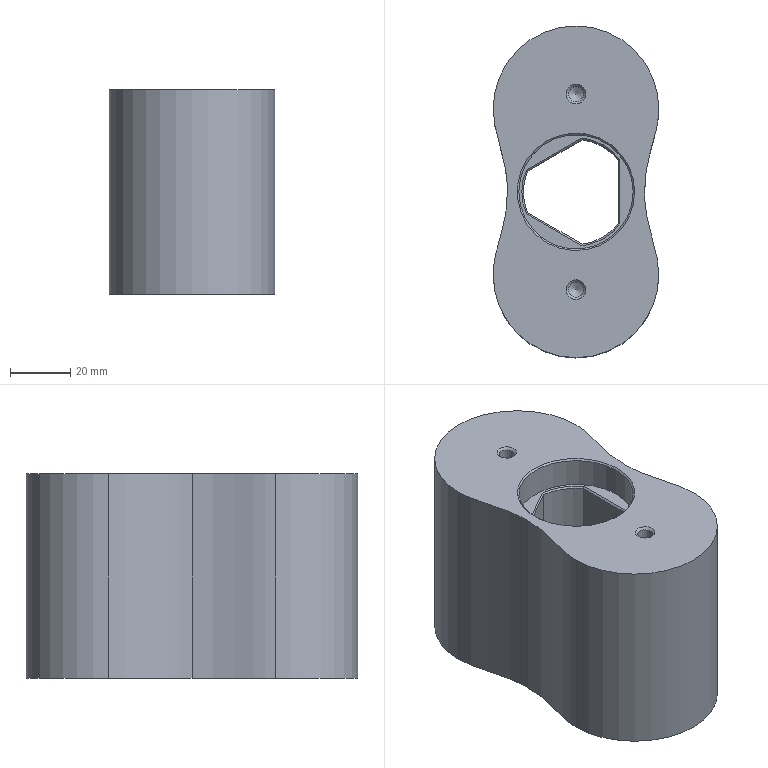Part | 1 solid | 44 faces | box 55.004 x 110.159 x 68 mm | volume 288337 mm3 | cone 16 | plane 13 | cylinder 11 | spline 4 | commonest cylinder face diameters 35 x3 2.5 x2 5 x2 55.004 x2 36.6 x1 38 x1
STEP:
#1=CARTESIAN_POINT('',(-16.093,-6.874,-62.5));
#2=VERTEX_POINT('',#1);
#3=CARTESIAN_POINT('',(-16.093,-6.874,-10.7));
#4=VERTEX_POINT('',#3);
#5=CARTESIAN_POINT('',(-16.093,-6.874,-84.29));
#6=DIRECTION('',(0.,0.,1.));
#7=VECTOR('',#6,1000.);
#8=LINE('',#5,#7);
#9=EDGE_CURVE('',#2,#4,#8,.T.);
#10=ORIENTED_EDGE('',*,*,#9,.F.);
#11=CARTESIAN_POINT('',(-16.093,6.874,-62.5));
#12=VERTEX_POINT('',#11);
#13=CARTESIAN_POINT('',(0.,0.,-62.5));
#14=DIRECTION('',(0.,0.,1.));
#15=DIRECTION('',(1.,0.,0.));
#16=AXIS2_PLACEMENT_3D('',#13,#14,#15);
#17=CIRCLE('',#16,17.5);
#18=EDGE_CURVE('',#2,#12,#17,.F.);
#19=ORIENTED_EDGE('',*,*,#18,.T.);
#20=CARTESIAN_POINT('',(-16.093,6.874,-10.7));
#21=VERTEX_POINT('',#20);
#22=CARTESIAN_POINT('',(-16.093,6.874,-84.29));
#23=DIRECTION('',(0.,0.,1.));
#24=VECTOR('',#23,1000.);
#25=LINE('',#22,#24);
#26=EDGE_CURVE('',#12,#21,#25,.T.);
#27=ORIENTED_EDGE('',*,*,#26,.T.);
#28=CARTESIAN_POINT('',(0.,0.,-10.7));
#29=DIRECTION('',(0.,0.,-1.));
#30=DIRECTION('',(-1.,0.,0.));
#31=AXIS2_PLACEMENT_3D('',#28,#29,#30);
#32=CIRCLE('',#31,17.5);
#33=EDGE_CURVE('',#21,#4,#32,.F.);
#34=ORIENTED_EDGE('',*,*,#33,.T.);
#35=EDGE_LOOP('',(#10,#19,#27,#34));
#36=FACE_BOUND('',#35,.T.);
#37=CARTESIAN_POINT('',(0.,0.,-68.));
#38=DIRECTION('',(0.,0.,-1.));
#39=DIRECTION('',(-1.,0.,0.));
#40=AXIS2_PLACEMENT_3D('',#37,#38,#39);
#41=CYLINDRICAL_SURFACE('',#40,17.5);
#42=ADVANCED_FACE('',(#36),#41,.F.);
#43=CARTESIAN_POINT('',(14.,-10.5,-62.5));
#44=VERTEX_POINT('',#43);
#45=CARTESIAN_POINT('',(14.,-10.5,-10.7));
#46=VERTEX_POINT('',#45);
#47=CARTESIAN_POINT('',(14.,-10.5,-84.29));
#48=DIRECTION('',(0.,0.,1.));
#49=VECTOR('',#48,1000.);
#50=LINE('',#47,#49);
#51=EDGE_CURVE('',#44,#46,#50,.T.);
#52=ORIENTED_EDGE('',*,*,#51,.F.);
#53=CARTESIAN_POINT('',(2.093,-17.374,-62.5));
#54=VERTEX_POINT('',#53);
#55=CARTESIAN_POINT('',(0.,0.,-62.5));
#56=DIRECTION('',(0.,0.,1.));
#57=DIRECTION('',(1.,0.,0.));
#58=AXIS2_PLACEMENT_3D('',#55,#56,#57);
#59=CIRCLE('',#58,17.5);
#60=EDGE_CURVE('',#44,#54,#59,.F.);
#61=ORIENTED_EDGE('',*,*,#60,.T.);
#62=CARTESIAN_POINT('',(2.093,-17.374,-10.7));
#63=VERTEX_POINT('',#62);
#64=CARTESIAN_POINT('',(2.093,-17.374,-84.29));
#65=DIRECTION('',(0.,0.,1.));
#66=VECTOR('',#65,1000.);
#67=LINE('',#64,#66);
#68=EDGE_CURVE('',#54,#63,#67,.T.);
#69=ORIENTED_EDGE('',*,*,#68,.T.);
#70=CARTESIAN_POINT('',(0.,0.,-10.7));
#71=DIRECTION('',(0.,0.,-1.));
#72=DIRECTION('',(-1.,0.,0.));
#73=AXIS2_PLACEMENT_3D('',#70,#71,#72);
#74=CIRCLE('',#73,17.5);
#75=EDGE_CURVE('',#63,#46,#74,.F.);
#76=ORIENTED_EDGE('',*,*,#75,.T.);
#77=EDGE_LOOP('',(#52,#61,#69,#76));
#78=FACE_BOUND('',#77,.T.);
#79=CARTESIAN_POINT('',(0.,0.,-68.));
#80=DIRECTION('',(0.,0.,-1.));
#81=DIRECTION('',(-1.,0.,0.));
#82=AXIS2_PLACEMENT_3D('',#79,#80,#81);
#83=CYLINDRICAL_SURFACE('',#82,17.5);
#84=ADVANCED_FACE('',(#78),#83,.F.);
#85=CARTESIAN_POINT('',(22.771,0.,-68.));
#86=VERTEX_POINT('',#85);
#87=CARTESIAN_POINT('',(27.502,27.577,-68.));
#88=VERTEX_POINT('',#87);
#89=CARTESIAN_POINT('',(22.771,0.,-68.));
#90=CARTESIAN_POINT('',(22.774,2.342,-68.));
#91=CARTESIAN_POINT('',(23.15,7.01,-68.));
#92=CARTESIAN_POINT('',(24.739,13.854,-68.));
#93=CARTESIAN_POINT('',(26.839,20.572,-68.));
#94=CARTESIAN_POINT('',(27.5,25.2,-68.));
#95=CARTESIAN_POINT('',(27.502,27.577,-68.));
#96=B_SPLINE_CURVE_WITH_KNOTS('',3,(#89,#90,#91,#92,#93,#94,#95),.UNSPECIFIED.,.F.,.F.,(4,1,1,1,4),(0.,0.007005,0.01401,0.02102,0.02802),.UNSPECIFIED.);
#97=EDGE_CURVE('',#86,#88,#96,.T.);
#98=ORIENTED_EDGE('',*,*,#97,.T.);
#99=CARTESIAN_POINT('',(27.502,27.577,0.));
#100=VERTEX_POINT('',#99);
#101=CARTESIAN_POINT('',(27.502,27.577,0.));
#102=CARTESIAN_POINT('',(27.502,27.577,-22.667));
#103=CARTESIAN_POINT('',(27.502,27.577,-45.333));
#104=CARTESIAN_POINT('',(27.502,27.577,-68.));
#105=B_SPLINE_CURVE_WITH_KNOTS('',3,(#101,#102,#103,#104),.UNSPECIFIED.,.F.,.F.,(4,4),(0.,1.),.UNSPECIFIED.);
#106=EDGE_CURVE('',#100,#88,#105,.T.);
#107=ORIENTED_EDGE('',*,*,#106,.F.);
#108=CARTESIAN_POINT('',(22.771,0.,0.));
#109=VERTEX_POINT('',#108);
#110=CARTESIAN_POINT('',(22.771,0.,0.));
#111=CARTESIAN_POINT('',(22.774,2.342,0.));
#112=CARTESIAN_POINT('',(23.15,7.01,0.));
#113=CARTESIAN_POINT('',(24.739,13.854,0.));
#114=CARTESIAN_POINT('',(26.839,20.572,0.));
#115=CARTESIAN_POINT('',(27.5,25.2,0.));
#116=CARTESIAN_POINT('',(27.502,27.577,0.));
#117=B_SPLINE_CURVE_WITH_KNOTS('',3,(#110,#111,#112,#113,#114,#115,#116),.UNSPECIFIED.,.F.,.F.,(4,1,1,1,4),(0.,0.007005,0.01401,0.02102,0.02802),.UNSPECIFIED.);
#118=EDGE_CURVE('',#109,#100,#117,.T.);
#119=ORIENTED_EDGE('',*,*,#118,.F.);
#120=CARTESIAN_POINT('',(22.771,0.,0.));
#121=DIRECTION('',(0.,0.,-1.));
#122=VECTOR('',#121,1000.);
#123=LINE('',#120,#122);
#124=EDGE_CURVE('',#109,#86,#123,.T.);
#125=ORIENTED_EDGE('',*,*,#124,.T.);
#126=EDGE_LOOP('',(#98,#107,#119,#125));
#127=FACE_BOUND('',#126,.T.);
#128=CARTESIAN_POINT('',(22.771,0.,0.));
#129=CARTESIAN_POINT('',(22.771,0.,-68.));
#130=CARTESIAN_POINT('',(22.774,2.34,0.));
#131=CARTESIAN_POINT('',(22.774,2.34,-68.));
#132=CARTESIAN_POINT('',(23.153,7.034,0.));
#133=CARTESIAN_POINT('',(23.153,7.034,-68.));
#134=CARTESIAN_POINT('',(24.749,13.889,0.));
#135=CARTESIAN_POINT('',(24.749,13.889,-68.));
#136=CARTESIAN_POINT('',(26.848,20.598,0.));
#137=CARTESIAN_POINT('',(26.848,20.598,-68.));
#138=CARTESIAN_POINT('',(27.5,25.237,0.));
#139=CARTESIAN_POINT('',(27.5,25.237,-68.));
#140=CARTESIAN_POINT('',(27.502,27.577,0.));
#141=CARTESIAN_POINT('',(27.502,27.577,-68.));
#142=B_SPLINE_SURFACE_WITH_KNOTS('',3,1,((#128,#129),(#130,#131),(#132,#133),(#134,#135),(#136,#137),(#138,#139),(#140,#141)),.SURF_OF_LINEAR_EXTRUSION.,.F.,.F.,.F.,(4,1,1,1,4),(2,2),(-0.000004078,0.25,0.5,0.75,1.),(0.,1.),.UNSPECIFIED.);
#143=ADVANCED_FACE('',(#127),#142,.F.);
#144=CARTESIAN_POINT('',(-27.502,27.577,-68.));
#145=VERTEX_POINT('',#144);
#146=CARTESIAN_POINT('',(0.,27.577,-68.));
#147=DIRECTION('',(0.,0.,1.));
#148=DIRECTION('',(1.,0.,0.));
#149=AXIS2_PLACEMENT_3D('',#146,#147,#148);
#150=CIRCLE('',#149,27.502);
#151=EDGE_CURVE('',#88,#145,#150,.T.);
#152=ORIENTED_EDGE('',*,*,#151,.T.);
#153=CARTESIAN_POINT('',(-27.502,27.577,0.));
#154=VERTEX_POINT('',#153);
#155=CARTESIAN_POINT('',(-27.502,27.577,-68.));
#156=CARTESIAN_POINT('',(-27.502,27.577,-45.333));
#157=CARTESIAN_POINT('',(-27.502,27.577,-22.667));
#158=CARTESIAN_POINT('',(-27.502,27.577,0.));
#159=B_SPLINE_CURVE_WITH_KNOTS('',3,(#155,#156,#157,#158),.UNSPECIFIED.,.F.,.F.,(4,4),(0.,1.),.UNSPECIFIED.);
#160=EDGE_CURVE('',#154,#145,#159,.F.);
#161=ORIENTED_EDGE('',*,*,#160,.F.);
#162=CARTESIAN_POINT('',(0.,27.577,0.));
#163=DIRECTION('',(0.,0.,1.));
#164=DIRECTION('',(1.,0.,0.));
#165=AXIS2_PLACEMENT_3D('',#162,#163,#164);
#166=CIRCLE('',#165,27.502);
#167=EDGE_CURVE('',#100,#154,#166,.T.);
#168=ORIENTED_EDGE('',*,*,#167,.F.);
#169=ORIENTED_EDGE('',*,*,#106,.T.);
#170=EDGE_LOOP('',(#152,#161,#168,#169));
#171=FACE_BOUND('',#170,.T.);
#172=CARTESIAN_POINT('',(0.,27.577,0.));
#173=DIRECTION('',(0.,0.,-1.));
#174=DIRECTION('',(-1.,0.,0.));
#175=AXIS2_PLACEMENT_3D('',#172,#173,#174);
#176=CYLINDRICAL_SURFACE('',#175,27.502);
#177=ADVANCED_FACE('',(#171),#176,.T.);
#178=CARTESIAN_POINT('',(-22.771,0.,-68.));
#179=VERTEX_POINT('',#178);
#180=CARTESIAN_POINT('',(-27.502,27.577,-68.));
#181=CARTESIAN_POINT('',(-27.5,25.228,-68.));
#182=CARTESIAN_POINT('',(-26.847,20.595,-68.));
#183=CARTESIAN_POINT('',(-24.741,13.863,-68.));
#184=CARTESIAN_POINT('',(-23.149,7.002,-68.));
#185=CARTESIAN_POINT('',(-22.774,2.348,-68.));
#186=CARTESIAN_POINT('',(-22.771,0.,-68.));
#187=B_SPLINE_CURVE_WITH_KNOTS('',3,(#180,#181,#182,#183,#184,#185,#186),.UNSPECIFIED.,.F.,.F.,(4,1,1,1,4),(0.,0.006997,0.01399,0.02099,0.02799),.UNSPECIFIED.);
#188=EDGE_CURVE('',#145,#179,#187,.T.);
#189=ORIENTED_EDGE('',*,*,#188,.T.);
#190=CARTESIAN_POINT('',(-22.771,0.,0.));
#191=VERTEX_POINT('',#190);
#192=CARTESIAN_POINT('',(-22.771,0.,0.));
#193=DIRECTION('',(0.,0.,-1.));
#194=VECTOR('',#193,1000.);
#195=LINE('',#192,#194);
#196=EDGE_CURVE('',#191,#179,#195,.T.);
#197=ORIENTED_EDGE('',*,*,#196,.F.);
#198=CARTESIAN_POINT('',(-27.502,27.577,0.));
#199=CARTESIAN_POINT('',(-27.5,25.228,0.));
#200=CARTESIAN_POINT('',(-26.847,20.595,0.));
#201=CARTESIAN_POINT('',(-24.741,13.863,0.));
#202=CARTESIAN_POINT('',(-23.149,7.002,0.));
#203=CARTESIAN_POINT('',(-22.774,2.348,0.));
#204=CARTESIAN_POINT('',(-22.771,0.,0.));
#205=B_SPLINE_CURVE_WITH_KNOTS('',3,(#198,#199,#200,#201,#202,#203,#204),.UNSPECIFIED.,.F.,.F.,(4,1,1,1,4),(0.,0.006997,0.01399,0.02099,0.02799),.UNSPECIFIED.);
#206=EDGE_CURVE('',#154,#191,#205,.T.);
#207=ORIENTED_EDGE('',*,*,#206,.F.);
#208=ORIENTED_EDGE('',*,*,#160,.T.);
#209=EDGE_LOOP('',(#189,#197,#207,#208));
#210=FACE_BOUND('',#209,.T.);
#211=CARTESIAN_POINT('',(-27.502,27.577,0.));
#212=CARTESIAN_POINT('',(-27.502,27.577,-68.));
#213=CARTESIAN_POINT('',(-27.5,25.237,0.));
#214=CARTESIAN_POINT('',(-27.5,25.237,-68.));
#215=CARTESIAN_POINT('',(-26.848,20.598,0.));
#216=CARTESIAN_POINT('',(-26.848,20.598,-68.));
#217=CARTESIAN_POINT('',(-24.749,13.889,0.));
#218=CARTESIAN_POINT('',(-24.749,13.889,-68.));
#219=CARTESIAN_POINT('',(-23.153,7.034,0.));
#220=CARTESIAN_POINT('',(-23.153,7.034,-68.));
#221=CARTESIAN_POINT('',(-22.774,2.34,0.));
#222=CARTESIAN_POINT('',(-22.774,2.34,-68.));
#223=CARTESIAN_POINT('',(-22.771,0.,0.));
#224=CARTESIAN_POINT('',(-22.771,0.,-68.));
#225=B_SPLINE_SURFACE_WITH_KNOTS('',3,1,((#211,#212),(#213,#214),(#215,#216),(#217,#218),(#219,#220),(#221,#222),(#223,#224)),.SURF_OF_LINEAR_EXTRUSION.,.F.,.F.,.F.,(4,1,1,1,4),(2,2),(0.,0.25,0.5,0.75,1.),(0.,1.),.UNSPECIFIED.);
#226=ADVANCED_FACE('',(#210),#225,.F.);
#227=CARTESIAN_POINT('',(-27.502,-27.577,-68.));
#228=VERTEX_POINT('',#227);
#229=CARTESIAN_POINT('',(-22.771,0.,-68.));
#230=CARTESIAN_POINT('',(-22.774,-2.342,-68.));
#231=CARTESIAN_POINT('',(-23.15,-7.01,-68.));
#232=CARTESIAN_POINT('',(-24.739,-13.854,-68.));
#233=CARTESIAN_POINT('',(-26.839,-20.572,-68.));
#234=CARTESIAN_POINT('',(-27.5,-25.2,-68.));
#235=CARTESIAN_POINT('',(-27.502,-27.577,-68.));
#236=B_SPLINE_CURVE_WITH_KNOTS('',3,(#229,#230,#231,#232,#233,#234,#235),.UNSPECIFIED.,.F.,.F.,(4,1,1,1,4),(0.,0.007005,0.01401,0.02102,0.02802),.UNSPECIFIED.);
#237=EDGE_CURVE('',#179,#228,#236,.T.);
#238=ORIENTED_EDGE('',*,*,#237,.T.);
#239=CARTESIAN_POINT('',(-27.502,-27.577,0.));
#240=VERTEX_POINT('',#239);
#241=CARTESIAN_POINT('',(-27.502,-27.577,0.));
#242=CARTESIAN_POINT('',(-27.502,-27.577,-22.667));
#243=CARTESIAN_POINT('',(-27.502,-27.577,-45.333));
#244=CARTESIAN_POINT('',(-27.502,-27.577,-68.));
#245=B_SPLINE_CURVE_WITH_KNOTS('',3,(#241,#242,#243,#244),.UNSPECIFIED.,.F.,.F.,(4,4),(0.,1.),.UNSPECIFIED.);
#246=EDGE_CURVE('',#240,#228,#245,.T.);
#247=ORIENTED_EDGE('',*,*,#246,.F.);
#248=CARTESIAN_POINT('',(-22.771,0.,0.));
#249=CARTESIAN_POINT('',(-22.774,-2.342,0.));
#250=CARTESIAN_POINT('',(-23.15,-7.01,0.));
#251=CARTESIAN_POINT('',(-24.739,-13.854,0.));
#252=CARTESIAN_POINT('',(-26.839,-20.572,0.));
#253=CARTESIAN_POINT('',(-27.5,-25.2,0.));
#254=CARTESIAN_POINT('',(-27.502,-27.577,0.));
#255=B_SPLINE_CURVE_WITH_KNOTS('',3,(#248,#249,#250,#251,#252,#253,#254),.UNSPECIFIED.,.F.,.F.,(4,1,1,1,4),(0.,0.007005,0.01401,0.02102,0.02802),.UNSPECIFIED.);
#256=EDGE_CURVE('',#191,#240,#255,.T.);
#257=ORIENTED_EDGE('',*,*,#256,.F.);
#258=ORIENTED_EDGE('',*,*,#196,.T.);
#259=EDGE_LOOP('',(#238,#247,#257,#258));
#260=FACE_BOUND('',#259,.T.);
#261=CARTESIAN_POINT('',(-22.771,0.,0.));
#262=CARTESIAN_POINT('',(-22.771,0.,-68.));
#263=CARTESIAN_POINT('',(-22.774,-2.34,0.));
#264=CARTESIAN_POINT('',(-22.774,-2.34,-68.));
#265=CARTESIAN_POINT('',(-23.153,-7.034,0.));
#266=CARTESIAN_POINT('',(-23.153,-7.034,-68.));
#267=CARTESIAN_POINT('',(-24.749,-13.889,0.));
#268=CARTESIAN_POINT('',(-24.749,-13.889,-68.));
#269=CARTESIAN_POINT('',(-26.848,-20.598,0.));
#270=CARTESIAN_POINT('',(-26.848,-20.598,-68.));
#271=CARTESIAN_POINT('',(-27.5,-25.237,0.));
#272=CARTESIAN_POINT('',(-27.5,-25.237,-68.));
#273=CARTESIAN_POINT('',(-27.502,-27.577,0.));
#274=CARTESIAN_POINT('',(-27.502,-27.577,-68.));
#275=B_SPLINE_SURFACE_WITH_KNOTS('',3,1,((#261,#262),(#263,#264),(#265,#266),(#267,#268),(#269,#270),(#271,#272),(#273,#274)),.SURF_OF_LINEAR_EXTRUSION.,.F.,.F.,.F.,(4,1,1,1,4),(2,2),(-0.000004078,0.25,0.5,0.75,1.),(0.,1.),.UNSPECIFIED.);
#276=ADVANCED_FACE('',(#260),#275,.F.);
#277=CARTESIAN_POINT('',(27.502,-27.577,-68.));
#278=VERTEX_POINT('',#277);
#279=CARTESIAN_POINT('',(0.,-27.577,-68.));
#280=DIRECTION('',(0.,0.,1.));
#281=DIRECTION('',(1.,0.,0.));
#282=AXIS2_PLACEMENT_3D('',#279,#280,#281);
#283=CIRCLE('',#282,27.502);
#284=EDGE_CURVE('',#228,#278,#283,.T.);
#285=ORIENTED_EDGE('',*,*,#284,.T.);
#286=CARTESIAN_POINT('',(27.502,-27.577,0.));
#287=VERTEX_POINT('',#286);
#288=CARTESIAN_POINT('',(27.502,-27.577,-68.));
#289=CARTESIAN_POINT('',(27.502,-27.577,-45.333));
#290=CARTESIAN_POINT('',(27.502,-27.577,-22.667));
#291=CARTESIAN_POINT('',(27.502,-27.577,0.));
#292=B_SPLINE_CURVE_WITH_KNOTS('',3,(#288,#289,#290,#291),.UNSPECIFIED.,.F.,.F.,(4,4),(0.,1.),.UNSPECIFIED.);
#293=EDGE_CURVE('',#287,#278,#292,.F.);
#294=ORIENTED_EDGE('',*,*,#293,.F.);
#295=CARTESIAN_POINT('',(0.,-27.577,0.));
#296=DIRECTION('',(0.,0.,1.));
#297=DIRECTION('',(1.,0.,0.));
#298=AXIS2_PLACEMENT_3D('',#295,#296,#297);
#299=CIRCLE('',#298,27.502);
#300=EDGE_CURVE('',#240,#287,#299,.T.);
#301=ORIENTED_EDGE('',*,*,#300,.F.);
#302=ORIENTED_EDGE('',*,*,#246,.T.);
#303=EDGE_LOOP('',(#285,#294,#301,#302));
#304=FACE_BOUND('',#303,.T.);
#305=CARTESIAN_POINT('',(0.,-27.577,0.));
#306=DIRECTION('',(0.,0.,-1.));
#307=DIRECTION('',(-1.,0.,0.));
#308=AXIS2_PLACEMENT_3D('',#305,#306,#307);
#309=CYLINDRICAL_SURFACE('',#308,27.502);
#310=ADVANCED_FACE('',(#304),#309,.T.);
#311=CARTESIAN_POINT('',(27.502,-27.577,-68.));
#312=CARTESIAN_POINT('',(27.5,-25.228,-68.));
#313=CARTESIAN_POINT('',(26.847,-20.595,-68.));
#314=CARTESIAN_POINT('',(24.741,-13.863,-68.));
#315=CARTESIAN_POINT('',(23.149,-7.002,-68.));
#316=CARTESIAN_POINT('',(22.774,-2.348,-68.));
#317=CARTESIAN_POINT('',(22.771,0.,-68.));
#318=B_SPLINE_CURVE_WITH_KNOTS('',3,(#311,#312,#313,#314,#315,#316,#317),.UNSPECIFIED.,.F.,.F.,(4,1,1,1,4),(0.,0.006997,0.01399,0.02099,0.02799),.UNSPECIFIED.);
#319=EDGE_CURVE('',#278,#86,#318,.T.);
#320=ORIENTED_EDGE('',*,*,#319,.T.);
#321=ORIENTED_EDGE('',*,*,#124,.F.);
#322=CARTESIAN_POINT('',(27.502,-27.577,0.));
#323=CARTESIAN_POINT('',(27.5,-25.228,0.));
#324=CARTESIAN_POINT('',(26.847,-20.595,0.));
#325=CARTESIAN_POINT('',(24.741,-13.863,0.));
#326=CARTESIAN_POINT('',(23.149,-7.002,0.));
#327=CARTESIAN_POINT('',(22.774,-2.348,0.));
#328=CARTESIAN_POINT('',(22.771,0.,0.));
#329=B_SPLINE_CURVE_WITH_KNOTS('',3,(#322,#323,#324,#325,#326,#327,#328),.UNSPECIFIED.,.F.,.F.,(4,1,1,1,4),(0.,0.006997,0.01399,0.02099,0.02799),.UNSPECIFIED.);
#330=EDGE_CURVE('',#287,#109,#329,.T.);
#331=ORIENTED_EDGE('',*,*,#330,.F.);
#332=ORIENTED_EDGE('',*,*,#293,.T.);
#333=EDGE_LOOP('',(#320,#321,#331,#332));
#334=FACE_BOUND('',#333,.T.);
#335=CARTESIAN_POINT('',(27.502,-27.577,0.));
#336=CARTESIAN_POINT('',(27.502,-27.577,-68.));
#337=CARTESIAN_POINT('',(27.5,-25.237,0.));
#338=CARTESIAN_POINT('',(27.5,-25.237,-68.));
#339=CARTESIAN_POINT('',(26.848,-20.598,0.));
#340=CARTESIAN_POINT('',(26.848,-20.598,-68.));
#341=CARTESIAN_POINT('',(24.749,-13.889,0.));
#342=CARTESIAN_POINT('',(24.749,-13.889,-68.));
#343=CARTESIAN_POINT('',(23.153,-7.034,0.));
#344=CARTESIAN_POINT('',(23.153,-7.034,-68.));
#345=CARTESIAN_POINT('',(22.774,-2.34,0.));
#346=CARTESIAN_POINT('',(22.774,-2.34,-68.));
#347=CARTESIAN_POINT('',(22.771,0.,0.));
#348=CARTESIAN_POINT('',(22.771,0.,-68.));
#349=B_SPLINE_SURFACE_WITH_KNOTS('',3,1,((#335,#336),(#337,#338),(#339,#340),(#341,#342),(#343,#344),(#345,#346),(#347,#348)),.SURF_OF_LINEAR_EXTRUSION.,.F.,.F.,.F.,(4,1,1,1,4),(2,2),(0.,0.25,0.5,0.75,1.),(0.,1.),.UNSPECIFIED.);
#350=ADVANCED_FACE('',(#334),#349,.F.);
#351=CARTESIAN_POINT('',(3.25,32.5,0.));
#352=VERTEX_POINT('',#351);
#353=CARTESIAN_POINT('',(0.,32.5,0.));
#354=DIRECTION('',(0.,0.,1.));
#355=DIRECTION('',(1.,0.,0.));
#356=AXIS2_PLACEMENT_3D('',#353,#354,#355);
#357=CIRCLE('',#356,3.25);
#358=EDGE_CURVE('',#352,#352,#357,.T.);
#359=ORIENTED_EDGE('',*,*,#358,.F.);
#360=EDGE_LOOP('',(#359));
#361=FACE_BOUND('',#360,.T.);
#362=CARTESIAN_POINT('',(3.25,-32.5,0.));
#363=VERTEX_POINT('',#362);
#364=CARTESIAN_POINT('',(0.,-32.5,0.));
#365=DIRECTION('',(0.,0.,1.));
#366=DIRECTION('',(1.,0.,0.));
#367=AXIS2_PLACEMENT_3D('',#364,#365,#366);
#368=CIRCLE('',#367,3.25);
#369=EDGE_CURVE('',#363,#363,#368,.T.);
#370=ORIENTED_EDGE('',*,*,#369,.F.);
#371=EDGE_LOOP('',(#370));
#372=FACE_BOUND('',#371,.T.);
#373=CARTESIAN_POINT('',(19.5,0.,0.));
#374=VERTEX_POINT('',#373);
#375=CARTESIAN_POINT('',(0.,0.,0.));
#376=DIRECTION('',(0.,0.,1.));
#377=DIRECTION('',(1.,0.,0.));
#378=AXIS2_PLACEMENT_3D('',#375,#376,#377);
#379=CIRCLE('',#378,19.5);
#380=EDGE_CURVE('',#374,#374,#379,.F.);
#381=ORIENTED_EDGE('',*,*,#380,.T.);
#382=EDGE_LOOP('',(#381));
#383=FACE_BOUND('',#382,.T.);
#384=ORIENTED_EDGE('',*,*,#118,.T.);
#385=ORIENTED_EDGE('',*,*,#167,.T.);
#386=ORIENTED_EDGE('',*,*,#206,.T.);
#387=ORIENTED_EDGE('',*,*,#256,.T.);
#388=ORIENTED_EDGE('',*,*,#300,.T.);
#389=ORIENTED_EDGE('',*,*,#330,.T.);
#390=EDGE_LOOP('',(#384,#385,#386,#387,#388,#389));
#391=FACE_BOUND('',#390,.T.);
#392=CARTESIAN_POINT('',(24.905,13.845,0.));
#393=DIRECTION('',(0.,0.,1.));
#394=DIRECTION('',(1.,0.,0.));
#395=AXIS2_PLACEMENT_3D('',#392,#393,#394);
#396=PLANE('',#395);
#397=ADVANCED_FACE('',(#361,#372,#383,#391),#396,.T.);
#398=CARTESIAN_POINT('',(-1.35,20.25,-68.));
#399=VERTEX_POINT('',#398);
#400=CARTESIAN_POINT('',(0.,20.25,-68.));
#401=DIRECTION('',(0.,0.,-1.));
#402=DIRECTION('',(-1.,0.,0.));
#403=AXIS2_PLACEMENT_3D('',#400,#401,#402);
#404=CIRCLE('',#403,1.35);
#405=EDGE_CURVE('',#399,#399,#404,.T.);
#406=ORIENTED_EDGE('',*,*,#405,.F.);
#407=EDGE_LOOP('',(#406));
#408=FACE_BOUND('',#407,.T.);
#409=CARTESIAN_POINT('',(-1.35,-20.25,-68.));
#410=VERTEX_POINT('',#409);
#411=CARTESIAN_POINT('',(0.,-20.25,-68.));
#412=DIRECTION('',(0.,0.,-1.));
#413=DIRECTION('',(-1.,0.,0.));
#414=AXIS2_PLACEMENT_3D('',#411,#412,#413);
#415=CIRCLE('',#414,1.35);
#416=EDGE_CURVE('',#410,#410,#415,.T.);
#417=ORIENTED_EDGE('',*,*,#416,.F.);
#418=EDGE_LOOP('',(#417));
#419=FACE_BOUND('',#418,.T.);
#420=CARTESIAN_POINT('',(18.8,0.,-68.));
#421=VERTEX_POINT('',#420);
#422=CARTESIAN_POINT('',(0.,0.,-68.));
#423=DIRECTION('',(0.,0.,1.));
#424=DIRECTION('',(1.,0.,0.));
#425=AXIS2_PLACEMENT_3D('',#422,#423,#424);
#426=CIRCLE('',#425,18.8);
#427=EDGE_CURVE('',#421,#421,#426,.T.);
#428=ORIENTED_EDGE('',*,*,#427,.T.);
#429=EDGE_LOOP('',(#428));
#430=FACE_BOUND('',#429,.T.);
#431=ORIENTED_EDGE('',*,*,#97,.F.);
#432=ORIENTED_EDGE('',*,*,#319,.F.);
#433=ORIENTED_EDGE('',*,*,#284,.F.);
#434=ORIENTED_EDGE('',*,*,#237,.F.);
#435=ORIENTED_EDGE('',*,*,#188,.F.);
#436=ORIENTED_EDGE('',*,*,#151,.F.);
#437=EDGE_LOOP('',(#431,#432,#433,#434,#435,#436));
#438=FACE_BOUND('',#437,.T.);
#439=CARTESIAN_POINT('',(24.905,13.845,-68.));
#440=DIRECTION('',(0.,0.,1.));
#441=DIRECTION('',(1.,0.,0.));
#442=AXIS2_PLACEMENT_3D('',#439,#440,#441);
#443=PLANE('',#442);
#444=ADVANCED_FACE('',(#408,#419,#430,#438),#443,.F.);
#445=CARTESIAN_POINT('',(19.,0.,-0.5));
#446=VERTEX_POINT('',#445);
#447=CARTESIAN_POINT('',(0.,0.,-0.5));
#448=DIRECTION('',(0.,0.,1.));
#449=DIRECTION('',(1.,0.,0.));
#450=AXIS2_PLACEMENT_3D('',#447,#448,#449);
#451=CIRCLE('',#450,19.);
#452=EDGE_CURVE('',#446,#446,#451,.T.);
#453=ORIENTED_EDGE('',*,*,#452,.T.);
#454=EDGE_LOOP('',(#453));
#455=FACE_BOUND('',#454,.T.);
#456=CARTESIAN_POINT('',(-19.,0.,-10.2));
#457=VERTEX_POINT('',#456);
#458=CARTESIAN_POINT('',(0.,0.,-10.2));
#459=DIRECTION('',(0.,0.,-1.));
#460=DIRECTION('',(-1.,0.,0.));
#461=AXIS2_PLACEMENT_3D('',#458,#459,#460);
#462=CIRCLE('',#461,19.);
#463=EDGE_CURVE('',#457,#457,#462,.T.);
#464=ORIENTED_EDGE('',*,*,#463,.T.);
#465=EDGE_LOOP('',(#464));
#466=FACE_BOUND('',#465,.T.);
#467=CARTESIAN_POINT('',(0.,0.,-68.));
#468=DIRECTION('',(0.,0.,-1.));
#469=DIRECTION('',(-1.,0.,0.));
#470=AXIS2_PLACEMENT_3D('',#467,#468,#469);
#471=CYLINDRICAL_SURFACE('',#470,19.);
#472=ADVANCED_FACE('',(#455,#466),#471,.F.);
#473=CARTESIAN_POINT('',(1.986,-17.89,-10.2));
#474=VERTEX_POINT('',#473);
#475=CARTESIAN_POINT('',(-16.486,-7.225,-10.2));
#476=VERTEX_POINT('',#475);
#477=CARTESIAN_POINT('',(-16.343,-7.307,-10.2));
#478=DIRECTION('',(-0.866,0.5,0.));
#479=VECTOR('',#478,1000.);
#480=LINE('',#477,#479);
#481=EDGE_CURVE('',#474,#476,#480,.T.);
#482=ORIENTED_EDGE('',*,*,#481,.T.);
#483=CARTESIAN_POINT('',(-16.486,7.225,-10.2));
#484=VERTEX_POINT('',#483);
#485=CARTESIAN_POINT('',(0.,0.,-10.2));
#486=DIRECTION('',(0.,0.,-1.));
#487=DIRECTION('',(-1.,0.,0.));
#488=AXIS2_PLACEMENT_3D('',#485,#486,#487);
#489=CIRCLE('',#488,18.);
#490=EDGE_CURVE('',#476,#484,#489,.T.);
#491=ORIENTED_EDGE('',*,*,#490,.T.);
#492=CARTESIAN_POINT('',(1.986,17.89,-10.2));
#493=VERTEX_POINT('',#492);
#494=CARTESIAN_POINT('',(1.843,17.807,-10.2));
#495=DIRECTION('',(0.866,0.5,0.));
#496=VECTOR('',#495,1000.);
#497=LINE('',#494,#496);
#498=EDGE_CURVE('',#484,#493,#497,.T.);
#499=ORIENTED_EDGE('',*,*,#498,.T.);
#500=CARTESIAN_POINT('',(14.5,10.665,-10.2));
#501=VERTEX_POINT('',#500);
#502=CARTESIAN_POINT('',(0.,0.,-10.2));
#503=DIRECTION('',(0.,0.,-1.));
#504=DIRECTION('',(-1.,0.,0.));
#505=AXIS2_PLACEMENT_3D('',#502,#503,#504);
#506=CIRCLE('',#505,18.);
#507=EDGE_CURVE('',#493,#501,#506,.T.);
#508=ORIENTED_EDGE('',*,*,#507,.T.);
#509=CARTESIAN_POINT('',(14.5,-10.665,-10.2));
#510=VERTEX_POINT('',#509);
#511=CARTESIAN_POINT('',(14.5,-10.5,-10.2));
#512=DIRECTION('',(0.,-1.,0.));
#513=VECTOR('',#512,1000.);
#514=LINE('',#511,#513);
#515=EDGE_CURVE('',#501,#510,#514,.T.);
#516=ORIENTED_EDGE('',*,*,#515,.T.);
#517=CARTESIAN_POINT('',(0.,0.,-10.2));
#518=DIRECTION('',(0.,0.,-1.));
#519=DIRECTION('',(-1.,0.,0.));
#520=AXIS2_PLACEMENT_3D('',#517,#518,#519);
#521=CIRCLE('',#520,18.);
#522=EDGE_CURVE('',#510,#474,#521,.T.);
#523=ORIENTED_EDGE('',*,*,#522,.T.);
#524=EDGE_LOOP('',(#482,#491,#499,#508,#516,#523));
#525=FACE_BOUND('',#524,.T.);
#526=ORIENTED_EDGE('',*,*,#463,.F.);
#527=EDGE_LOOP('',(#526));
#528=FACE_BOUND('',#527,.T.);
#529=CARTESIAN_POINT('',(0.,19.,-10.2));
#530=DIRECTION('',(0.,0.,-1.));
#531=DIRECTION('',(-1.,0.,0.));
#532=AXIS2_PLACEMENT_3D('',#529,#530,#531);
#533=PLANE('',#532);
#534=ADVANCED_FACE('',(#525,#528),#533,.F.);
#535=CARTESIAN_POINT('',(2.093,17.374,-62.5));
#536=VERTEX_POINT('',#535);
#537=CARTESIAN_POINT('',(2.093,17.374,-10.7));
#538=VERTEX_POINT('',#537);
#539=CARTESIAN_POINT('',(2.093,17.374,-84.29));
#540=DIRECTION('',(0.,0.,1.));
#541=VECTOR('',#540,1000.);
#542=LINE('',#539,#541);
#543=EDGE_CURVE('',#536,#538,#542,.T.);
#544=ORIENTED_EDGE('',*,*,#543,.F.);
#545=CARTESIAN_POINT('',(14.,10.5,-62.5));
#546=VERTEX_POINT('',#545);
#547=CARTESIAN_POINT('',(0.,0.,-62.5));
#548=DIRECTION('',(0.,0.,1.));
#549=DIRECTION('',(1.,0.,0.));
#550=AXIS2_PLACEMENT_3D('',#547,#548,#549);
#551=CIRCLE('',#550,17.5);
#552=EDGE_CURVE('',#536,#546,#551,.F.);
#553=ORIENTED_EDGE('',*,*,#552,.T.);
#554=CARTESIAN_POINT('',(14.,10.5,-10.7));
#555=VERTEX_POINT('',#554);
#556=CARTESIAN_POINT('',(14.,10.5,-84.29));
#557=DIRECTION('',(0.,0.,1.));
#558=VECTOR('',#557,1000.);
#559=LINE('',#556,#558);
#560=EDGE_CURVE('',#546,#555,#559,.T.);
#561=ORIENTED_EDGE('',*,*,#560,.T.);
#562=CARTESIAN_POINT('',(0.,0.,-10.7));
#563=DIRECTION('',(0.,0.,-1.));
#564=DIRECTION('',(-1.,0.,0.));
#565=AXIS2_PLACEMENT_3D('',#562,#563,#564);
#566=CIRCLE('',#565,17.5);
#567=EDGE_CURVE('',#555,#538,#566,.F.);
#568=ORIENTED_EDGE('',*,*,#567,.T.);
#569=EDGE_LOOP('',(#544,#553,#561,#568));
#570=FACE_BOUND('',#569,.T.);
#571=CARTESIAN_POINT('',(0.,0.,-68.));
#572=DIRECTION('',(0.,0.,-1.));
#573=DIRECTION('',(-1.,0.,0.));
#574=AXIS2_PLACEMENT_3D('',#571,#572,#573);
#575=CYLINDRICAL_SURFACE('',#574,17.5);
#576=ADVANCED_FACE('',(#570),#575,.F.);
#577=CARTESIAN_POINT('',(1.986,17.89,-63.));
#578=VERTEX_POINT('',#577);
#579=CARTESIAN_POINT('',(-16.486,7.225,-63.));
#580=VERTEX_POINT('',#579);
#581=CARTESIAN_POINT('',(-16.343,7.307,-63.));
#582=DIRECTION('',(-0.866,-0.5,0.));
#583=VECTOR('',#582,1000.);
#584=LINE('',#581,#583);
#585=EDGE_CURVE('',#578,#580,#584,.T.);
#586=ORIENTED_EDGE('',*,*,#585,.T.);
#587=CARTESIAN_POINT('',(-16.486,-7.225,-63.));
#588=VERTEX_POINT('',#587);
#589=CARTESIAN_POINT('',(0.,0.,-63.));
#590=DIRECTION('',(0.,0.,1.));
#591=DIRECTION('',(1.,0.,0.));
#592=AXIS2_PLACEMENT_3D('',#589,#590,#591);
#593=CIRCLE('',#592,18.);
#594=EDGE_CURVE('',#580,#588,#593,.T.);
#595=ORIENTED_EDGE('',*,*,#594,.T.);
#596=CARTESIAN_POINT('',(1.986,-17.89,-63.));
#597=VERTEX_POINT('',#596);
#598=CARTESIAN_POINT('',(1.843,-17.807,-63.));
#599=DIRECTION('',(0.866,-0.5,0.));
#600=VECTOR('',#599,1000.);
#601=LINE('',#598,#600);
#602=EDGE_CURVE('',#588,#597,#601,.T.);
#603=ORIENTED_EDGE('',*,*,#602,.T.);
#604=CARTESIAN_POINT('',(14.5,-10.665,-63.));
#605=VERTEX_POINT('',#604);
#606=CARTESIAN_POINT('',(0.,0.,-63.));
#607=DIRECTION('',(0.,0.,1.));
#608=DIRECTION('',(1.,0.,0.));
#609=AXIS2_PLACEMENT_3D('',#606,#607,#608);
#610=CIRCLE('',#609,18.);
#611=EDGE_CURVE('',#597,#605,#610,.T.);
#612=ORIENTED_EDGE('',*,*,#611,.T.);
#613=CARTESIAN_POINT('',(14.5,10.665,-63.));
#614=VERTEX_POINT('',#613);
#615=CARTESIAN_POINT('',(14.5,10.5,-63.));
#616=DIRECTION('',(0.,1.,0.));
#617=VECTOR('',#616,1000.);
#618=LINE('',#615,#617);
#619=EDGE_CURVE('',#605,#614,#618,.T.);
#620=ORIENTED_EDGE('',*,*,#619,.T.);
#621=CARTESIAN_POINT('',(0.,0.,-63.));
#622=DIRECTION('',(0.,0.,1.));
#623=DIRECTION('',(1.,0.,0.));
#624=AXIS2_PLACEMENT_3D('',#621,#622,#623);
#625=CIRCLE('',#624,18.);
#626=EDGE_CURVE('',#614,#578,#625,.T.);
#627=ORIENTED_EDGE('',*,*,#626,.T.);
#628=EDGE_LOOP('',(#586,#595,#603,#612,#620,#627));
#629=FACE_BOUND('',#628,.T.);
#630=CARTESIAN_POINT('',(-18.3,0.,-63.));
#631=VERTEX_POINT('',#630);
#632=CARTESIAN_POINT('',(0.,0.,-63.));
#633=DIRECTION('',(0.,0.,-1.));
#634=DIRECTION('',(-1.,0.,0.));
#635=AXIS2_PLACEMENT_3D('',#632,#633,#634);
#636=CIRCLE('',#635,18.3);
#637=EDGE_CURVE('',#631,#631,#636,.T.);
#638=ORIENTED_EDGE('',*,*,#637,.T.);
#639=EDGE_LOOP('',(#638));
#640=FACE_BOUND('',#639,.T.);
#641=CARTESIAN_POINT('',(0.,17.5,-63.));
#642=DIRECTION('',(0.,0.,1.));
#643=DIRECTION('',(1.,0.,0.));
#644=AXIS2_PLACEMENT_3D('',#641,#642,#643);
#645=PLANE('',#644);
#646=ADVANCED_FACE('',(#629,#640),#645,.F.);
#647=CARTESIAN_POINT('',(18.3,0.,-67.5));
#648=VERTEX_POINT('',#647);
#649=CARTESIAN_POINT('',(0.,0.,-67.5));
#650=DIRECTION('',(0.,0.,1.));
#651=DIRECTION('',(1.,0.,0.));
#652=AXIS2_PLACEMENT_3D('',#649,#650,#651);
#653=CIRCLE('',#652,18.3);
#654=EDGE_CURVE('',#648,#648,#653,.F.);
#655=ORIENTED_EDGE('',*,*,#654,.T.);
#656=EDGE_LOOP('',(#655));
#657=FACE_BOUND('',#656,.T.);
#658=ORIENTED_EDGE('',*,*,#637,.F.);
#659=EDGE_LOOP('',(#658));
#660=FACE_BOUND('',#659,.T.);
#661=CARTESIAN_POINT('',(0.,0.,-68.));
#662=DIRECTION('',(0.,0.,-1.));
#663=DIRECTION('',(-1.,0.,0.));
#664=AXIS2_PLACEMENT_3D('',#661,#662,#663);
#665=CYLINDRICAL_SURFACE('',#664,18.3);
#666=ADVANCED_FACE('',(#657,#660),#665,.F.);
#667=ORIENTED_EDGE('',*,*,#560,.F.);
#668=CARTESIAN_POINT('',(14.,-10.5,-62.5));
#669=DIRECTION('',(0.,-1.,0.));
#670=VECTOR('',#669,1000.);
#671=LINE('',#668,#670);
#672=EDGE_CURVE('',#546,#44,#671,.T.);
#673=ORIENTED_EDGE('',*,*,#672,.T.);
#674=ORIENTED_EDGE('',*,*,#51,.T.);
#675=CARTESIAN_POINT('',(14.,10.5,-10.7));
#676=DIRECTION('',(0.,1.,0.));
#677=VECTOR('',#676,1000.);
#678=LINE('',#675,#677);
#679=EDGE_CURVE('',#46,#555,#678,.T.);
#680=ORIENTED_EDGE('',*,*,#679,.T.);
#681=EDGE_LOOP('',(#667,#673,#674,#680));
#682=FACE_BOUND('',#681,.T.);
#683=CARTESIAN_POINT('',(14.,10.5,-84.29));
#684=DIRECTION('',(-1.,0.,0.));
#685=DIRECTION('',(0.,0.,1.));
#686=AXIS2_PLACEMENT_3D('',#683,#684,#685);
#687=PLANE('',#686);
#688=ADVANCED_FACE('',(#682),#687,.T.);
#689=ORIENTED_EDGE('',*,*,#68,.F.);
#690=CARTESIAN_POINT('',(-16.093,-6.874,-62.5));
#691=DIRECTION('',(-0.866,0.5,0.));
#692=VECTOR('',#691,1000.);
#693=LINE('',#690,#692);
#694=EDGE_CURVE('',#54,#2,#693,.T.);
#695=ORIENTED_EDGE('',*,*,#694,.T.);
#696=ORIENTED_EDGE('',*,*,#9,.T.);
#697=CARTESIAN_POINT('',(2.093,-17.374,-10.7));
#698=DIRECTION('',(0.866,-0.5,0.));
#699=VECTOR('',#698,1000.);
#700=LINE('',#697,#699);
#701=EDGE_CURVE('',#4,#63,#700,.T.);
#702=ORIENTED_EDGE('',*,*,#701,.T.);
#703=EDGE_LOOP('',(#689,#695,#696,#702));
#704=FACE_BOUND('',#703,.T.);
#705=CARTESIAN_POINT('',(2.093,-17.374,-84.29));
#706=DIRECTION('',(0.5,0.866,0.));
#707=DIRECTION('',(-0.866,0.5,0.));
#708=AXIS2_PLACEMENT_3D('',#705,#706,#707);
#709=PLANE('',#708);
#710=ADVANCED_FACE('',(#704),#709,.T.);
#711=ORIENTED_EDGE('',*,*,#26,.F.);
#712=CARTESIAN_POINT('',(2.093,17.374,-62.5));
#713=DIRECTION('',(0.866,0.5,0.));
#714=VECTOR('',#713,1000.);
#715=LINE('',#712,#714);
#716=EDGE_CURVE('',#12,#536,#715,.T.);
#717=ORIENTED_EDGE('',*,*,#716,.T.);
#718=ORIENTED_EDGE('',*,*,#543,.T.);
#719=CARTESIAN_POINT('',(-16.093,6.874,-10.7));
#720=DIRECTION('',(-0.866,-0.5,0.));
#721=VECTOR('',#720,1000.);
#722=LINE('',#719,#721);
#723=EDGE_CURVE('',#538,#21,#722,.T.);
#724=ORIENTED_EDGE('',*,*,#723,.T.);
#725=EDGE_LOOP('',(#711,#717,#718,#724));
#726=FACE_BOUND('',#725,.T.);
#727=CARTESIAN_POINT('',(-16.093,6.874,-84.29));
#728=DIRECTION('',(0.5,-0.866,0.));
#729=DIRECTION('',(0.866,0.5,0.));
#730=AXIS2_PLACEMENT_3D('',#727,#728,#729);
#731=PLANE('',#730);
#732=ADVANCED_FACE('',(#726),#731,.T.);
#733=ORIENTED_EDGE('',*,*,#452,.F.);
#734=EDGE_LOOP('',(#733));
#735=FACE_BOUND('',#734,.T.);
#736=ORIENTED_EDGE('',*,*,#380,.F.);
#737=EDGE_LOOP('',(#736));
#738=FACE_BOUND('',#737,.T.);
#739=CARTESIAN_POINT('',(0.,0.,0.));
#740=DIRECTION('',(0.,0.,1.));
#741=DIRECTION('',(1.,0.,0.));
#742=AXIS2_PLACEMENT_3D('',#739,#740,#741);
#743=CONICAL_SURFACE('',#742,19.5,0.7854);
#744=ADVANCED_FACE('',(#735,#738),#743,.F.);
#745=ORIENTED_EDGE('',*,*,#427,.F.);
#746=EDGE_LOOP('',(#745));
#747=FACE_BOUND('',#746,.T.);
#748=ORIENTED_EDGE('',*,*,#654,.F.);
#749=EDGE_LOOP('',(#748));
#750=FACE_BOUND('',#749,.T.);
#751=CARTESIAN_POINT('',(0.,0.,-67.5));
#752=DIRECTION('',(0.,0.,-1.));
#753=DIRECTION('',(-1.,0.,0.));
#754=AXIS2_PLACEMENT_3D('',#751,#752,#753);
#755=CONICAL_SURFACE('',#754,18.3,0.7854);
#756=ADVANCED_FACE('',(#747,#750),#755,.F.);
#757=CARTESIAN_POINT('',(14.,10.5,-62.5));
#758=CARTESIAN_POINT('',(14.167,10.556,-62.667));
#759=CARTESIAN_POINT('',(14.333,10.611,-62.833));
#760=CARTESIAN_POINT('',(14.5,10.665,-63.));
#761=B_SPLINE_CURVE_WITH_KNOTS('',3,(#757,#758,#759,#760),.UNSPECIFIED.,.F.,.F.,(4,4),(0.,0.0007262),.UNSPECIFIED.);
#762=EDGE_CURVE('',#614,#546,#761,.F.);
#763=ORIENTED_EDGE('',*,*,#762,.F.);
#764=ORIENTED_EDGE('',*,*,#619,.F.);
#765=CARTESIAN_POINT('',(14.,-10.5,-62.5));
#766=CARTESIAN_POINT('',(14.167,-10.556,-62.667));
#767=CARTESIAN_POINT('',(14.333,-10.611,-62.833));
#768=CARTESIAN_POINT('',(14.5,-10.665,-63.));
#769=B_SPLINE_CURVE_WITH_KNOTS('',3,(#765,#766,#767,#768),.UNSPECIFIED.,.F.,.F.,(4,4),(0.,0.0007262),.UNSPECIFIED.);
#770=EDGE_CURVE('',#44,#605,#769,.T.);
#771=ORIENTED_EDGE('',*,*,#770,.F.);
#772=ORIENTED_EDGE('',*,*,#672,.F.);
#773=EDGE_LOOP('',(#763,#764,#771,#772));
#774=FACE_BOUND('',#773,.T.);
#775=CARTESIAN_POINT('',(14.5,17.5,-63.));
#776=DIRECTION('',(-0.7071,0.,-0.7071));
#777=DIRECTION('',(0.,-1.,0.));
#778=AXIS2_PLACEMENT_3D('',#775,#776,#777);
#779=PLANE('',#778);
#780=ADVANCED_FACE('',(#774),#779,.T.);
#781=ORIENTED_EDGE('',*,*,#770,.T.);
#782=ORIENTED_EDGE('',*,*,#611,.F.);
#783=CARTESIAN_POINT('',(2.093,-17.374,-62.5));
#784=CARTESIAN_POINT('',(2.058,-17.546,-62.667));
#785=CARTESIAN_POINT('',(2.022,-17.718,-62.833));
#786=CARTESIAN_POINT('',(1.986,-17.89,-63.));
#787=B_SPLINE_CURVE_WITH_KNOTS('',3,(#783,#784,#785,#786),.UNSPECIFIED.,.F.,.F.,(4,4),(0.,0.0007262),.UNSPECIFIED.);
#788=EDGE_CURVE('',#54,#597,#787,.T.);
#789=ORIENTED_EDGE('',*,*,#788,.F.);
#790=ORIENTED_EDGE('',*,*,#60,.F.);
#791=EDGE_LOOP('',(#781,#782,#789,#790));
#792=FACE_BOUND('',#791,.T.);
#793=CARTESIAN_POINT('',(0.,0.,-62.5));
#794=DIRECTION('',(0.,0.,-1.));
#795=DIRECTION('',(-1.,0.,0.));
#796=AXIS2_PLACEMENT_3D('',#793,#794,#795);
#797=CONICAL_SURFACE('',#796,17.5,0.7854);
#798=ADVANCED_FACE('',(#792),#797,.F.);
#799=ORIENTED_EDGE('',*,*,#762,.T.);
#800=ORIENTED_EDGE('',*,*,#552,.F.);
#801=CARTESIAN_POINT('',(2.093,17.374,-62.5));
#802=CARTESIAN_POINT('',(2.058,17.546,-62.667));
#803=CARTESIAN_POINT('',(2.022,17.718,-62.833));
#804=CARTESIAN_POINT('',(1.986,17.89,-63.));
#805=B_SPLINE_CURVE_WITH_KNOTS('',3,(#801,#802,#803,#804),.UNSPECIFIED.,.F.,.F.,(4,4),(0.,0.0007262),.UNSPECIFIED.);
#806=EDGE_CURVE('',#578,#536,#805,.F.);
#807=ORIENTED_EDGE('',*,*,#806,.F.);
#808=ORIENTED_EDGE('',*,*,#626,.F.);
#809=EDGE_LOOP('',(#799,#800,#807,#808));
#810=FACE_BOUND('',#809,.T.);
#811=CARTESIAN_POINT('',(0.,0.,-62.5));
#812=DIRECTION('',(0.,0.,-1.));
#813=DIRECTION('',(-1.,0.,0.));
#814=AXIS2_PLACEMENT_3D('',#811,#812,#813);
#815=CONICAL_SURFACE('',#814,17.5,0.7854);
#816=ADVANCED_FACE('',(#810),#815,.F.);
#817=ORIENTED_EDGE('',*,*,#788,.T.);
#818=ORIENTED_EDGE('',*,*,#602,.F.);
#819=CARTESIAN_POINT('',(-16.486,-7.225,-63.));
#820=CARTESIAN_POINT('',(-16.356,-7.108,-62.833));
#821=CARTESIAN_POINT('',(-16.225,-6.991,-62.667));
#822=CARTESIAN_POINT('',(-16.093,-6.874,-62.5));
#823=B_SPLINE_CURVE_WITH_KNOTS('',3,(#819,#820,#821,#822),.UNSPECIFIED.,.F.,.F.,(4,4),(0.,0.0007262),.UNSPECIFIED.);
#824=EDGE_CURVE('',#2,#588,#823,.F.);
#825=ORIENTED_EDGE('',*,*,#824,.F.);
#826=ORIENTED_EDGE('',*,*,#694,.F.);
#827=EDGE_LOOP('',(#817,#818,#825,#826));
#828=FACE_BOUND('',#827,.T.);
#829=CARTESIAN_POINT('',(-14.828,-8.182,-63.));
#830=DIRECTION('',(0.3536,0.6124,-0.7071));
#831=DIRECTION('',(-0.866,0.5,0.));
#832=AXIS2_PLACEMENT_3D('',#829,#830,#831);
#833=PLANE('',#832);
#834=ADVANCED_FACE('',(#828),#833,.T.);
#835=ORIENTED_EDGE('',*,*,#806,.T.);
#836=ORIENTED_EDGE('',*,*,#716,.F.);
#837=CARTESIAN_POINT('',(-16.093,6.874,-62.5));
#838=CARTESIAN_POINT('',(-16.225,6.991,-62.667));
#839=CARTESIAN_POINT('',(-16.356,7.108,-62.833));
#840=CARTESIAN_POINT('',(-16.486,7.225,-63.));
#841=B_SPLINE_CURVE_WITH_KNOTS('',3,(#837,#838,#839,#840),.UNSPECIFIED.,.F.,.F.,(4,4),(0.,0.0007262),.UNSPECIFIED.);
#842=EDGE_CURVE('',#580,#12,#841,.F.);
#843=ORIENTED_EDGE('',*,*,#842,.F.);
#844=ORIENTED_EDGE('',*,*,#585,.F.);
#845=EDGE_LOOP('',(#835,#836,#843,#844));
#846=FACE_BOUND('',#845,.T.);
#847=CARTESIAN_POINT('',(0.3277,16.932,-63.));
#848=DIRECTION('',(0.3536,-0.6124,-0.7071));
#849=DIRECTION('',(0.866,0.5,0.));
#850=AXIS2_PLACEMENT_3D('',#847,#848,#849);
#851=PLANE('',#850);
#852=ADVANCED_FACE('',(#846),#851,.T.);
#853=ORIENTED_EDGE('',*,*,#824,.T.);
#854=ORIENTED_EDGE('',*,*,#594,.F.);
#855=ORIENTED_EDGE('',*,*,#842,.T.);
#856=ORIENTED_EDGE('',*,*,#18,.F.);
#857=EDGE_LOOP('',(#853,#854,#855,#856));
#858=FACE_BOUND('',#857,.T.);
#859=CARTESIAN_POINT('',(0.,0.,-62.5));
#860=DIRECTION('',(0.,0.,-1.));
#861=DIRECTION('',(-1.,0.,0.));
#862=AXIS2_PLACEMENT_3D('',#859,#860,#861);
#863=CONICAL_SURFACE('',#862,17.5,0.7854);
#864=ADVANCED_FACE('',(#858),#863,.F.);
#865=CARTESIAN_POINT('',(14.5,10.665,-10.2));
#866=CARTESIAN_POINT('',(14.333,10.611,-10.367));
#867=CARTESIAN_POINT('',(14.167,10.556,-10.533));
#868=CARTESIAN_POINT('',(14.,10.5,-10.7));
#869=B_SPLINE_CURVE_WITH_KNOTS('',3,(#865,#866,#867,#868),.UNSPECIFIED.,.F.,.F.,(4,4),(0.,0.0007262),.UNSPECIFIED.);
#870=EDGE_CURVE('',#555,#501,#869,.F.);
#871=ORIENTED_EDGE('',*,*,#870,.F.);
#872=ORIENTED_EDGE('',*,*,#679,.F.);
#873=CARTESIAN_POINT('',(14.5,-10.665,-10.2));
#874=CARTESIAN_POINT('',(14.333,-10.611,-10.367));
#875=CARTESIAN_POINT('',(14.167,-10.556,-10.533));
#876=CARTESIAN_POINT('',(14.,-10.5,-10.7));
#877=B_SPLINE_CURVE_WITH_KNOTS('',3,(#873,#874,#875,#876),.UNSPECIFIED.,.F.,.F.,(4,4),(0.,0.0007262),.UNSPECIFIED.);
#878=EDGE_CURVE('',#510,#46,#877,.T.);
#879=ORIENTED_EDGE('',*,*,#878,.F.);
#880=ORIENTED_EDGE('',*,*,#515,.F.);
#881=EDGE_LOOP('',(#871,#872,#879,#880));
#882=FACE_BOUND('',#881,.T.);
#883=CARTESIAN_POINT('',(14.5,19.,-10.2));
#884=DIRECTION('',(-0.7071,0.,0.7071));
#885=DIRECTION('',(0.,1.,0.));
#886=AXIS2_PLACEMENT_3D('',#883,#884,#885);
#887=PLANE('',#886);
#888=ADVANCED_FACE('',(#882),#887,.T.);
#889=ORIENTED_EDGE('',*,*,#878,.T.);
#890=ORIENTED_EDGE('',*,*,#75,.F.);
#891=CARTESIAN_POINT('',(1.986,-17.89,-10.2));
#892=CARTESIAN_POINT('',(2.022,-17.718,-10.367));
#893=CARTESIAN_POINT('',(2.058,-17.546,-10.533));
#894=CARTESIAN_POINT('',(2.093,-17.374,-10.7));
#895=B_SPLINE_CURVE_WITH_KNOTS('',3,(#891,#892,#893,#894),.UNSPECIFIED.,.F.,.F.,(4,4),(0.,0.0007262),.UNSPECIFIED.);
#896=EDGE_CURVE('',#474,#63,#895,.T.);
#897=ORIENTED_EDGE('',*,*,#896,.F.);
#898=ORIENTED_EDGE('',*,*,#522,.F.);
#899=EDGE_LOOP('',(#889,#890,#897,#898));
#900=FACE_BOUND('',#899,.T.);
#901=CARTESIAN_POINT('',(0.,0.,-10.2));
#902=DIRECTION('',(0.,0.,1.));
#903=DIRECTION('',(1.,0.,0.));
#904=AXIS2_PLACEMENT_3D('',#901,#902,#903);
#905=CONICAL_SURFACE('',#904,18.,0.7854);
#906=ADVANCED_FACE('',(#900),#905,.F.);
#907=ORIENTED_EDGE('',*,*,#870,.T.);
#908=ORIENTED_EDGE('',*,*,#507,.F.);
#909=CARTESIAN_POINT('',(1.986,17.89,-10.2));
#910=CARTESIAN_POINT('',(2.022,17.718,-10.367));
#911=CARTESIAN_POINT('',(2.058,17.546,-10.533));
#912=CARTESIAN_POINT('',(2.093,17.374,-10.7));
#913=B_SPLINE_CURVE_WITH_KNOTS('',3,(#909,#910,#911,#912),.UNSPECIFIED.,.F.,.F.,(4,4),(0.,0.0007262),.UNSPECIFIED.);
#914=EDGE_CURVE('',#538,#493,#913,.F.);
#915=ORIENTED_EDGE('',*,*,#914,.F.);
#916=ORIENTED_EDGE('',*,*,#567,.F.);
#917=EDGE_LOOP('',(#907,#908,#915,#916));
#918=FACE_BOUND('',#917,.T.);
#919=CARTESIAN_POINT('',(0.,0.,-10.2));
#920=DIRECTION('',(0.,0.,1.));
#921=DIRECTION('',(1.,0.,0.));
#922=AXIS2_PLACEMENT_3D('',#919,#920,#921);
#923=CONICAL_SURFACE('',#922,18.,0.7854);
#924=ADVANCED_FACE('',(#918),#923,.F.);
#925=ORIENTED_EDGE('',*,*,#896,.T.);
#926=ORIENTED_EDGE('',*,*,#701,.F.);
#927=CARTESIAN_POINT('',(-16.093,-6.874,-10.7));
#928=CARTESIAN_POINT('',(-16.225,-6.991,-10.533));
#929=CARTESIAN_POINT('',(-16.356,-7.108,-10.367));
#930=CARTESIAN_POINT('',(-16.486,-7.225,-10.2));
#931=B_SPLINE_CURVE_WITH_KNOTS('',3,(#927,#928,#929,#930),.UNSPECIFIED.,.F.,.F.,(4,4),(0.,0.0007262),.UNSPECIFIED.);
#932=EDGE_CURVE('',#476,#4,#931,.F.);
#933=ORIENTED_EDGE('',*,*,#932,.F.);
#934=ORIENTED_EDGE('',*,*,#481,.F.);
#935=EDGE_LOOP('',(#925,#926,#933,#934));
#936=FACE_BOUND('',#935,.T.);
#937=CARTESIAN_POINT('',(-15.477,-7.807,-10.2));
#938=DIRECTION('',(0.3536,0.6124,0.7071));
#939=DIRECTION('',(0.866,-0.5,0.));
#940=AXIS2_PLACEMENT_3D('',#937,#938,#939);
#941=PLANE('',#940);
#942=ADVANCED_FACE('',(#936),#941,.T.);
#943=ORIENTED_EDGE('',*,*,#914,.T.);
#944=ORIENTED_EDGE('',*,*,#498,.F.);
#945=CARTESIAN_POINT('',(-16.486,7.225,-10.2));
#946=CARTESIAN_POINT('',(-16.356,7.108,-10.367));
#947=CARTESIAN_POINT('',(-16.225,6.991,-10.533));
#948=CARTESIAN_POINT('',(-16.093,6.874,-10.7));
#949=B_SPLINE_CURVE_WITH_KNOTS('',3,(#945,#946,#947,#948),.UNSPECIFIED.,.F.,.F.,(4,4),(0.,0.0007262),.UNSPECIFIED.);
#950=EDGE_CURVE('',#21,#484,#949,.F.);
#951=ORIENTED_EDGE('',*,*,#950,.F.);
#952=ORIENTED_EDGE('',*,*,#723,.F.);
#953=EDGE_LOOP('',(#943,#944,#951,#952));
#954=FACE_BOUND('',#953,.T.);
#955=CARTESIAN_POINT('',(0.9772,17.307,-10.2));
#956=DIRECTION('',(0.3536,-0.6124,0.7071));
#957=DIRECTION('',(-0.866,-0.5,0.));
#958=AXIS2_PLACEMENT_3D('',#955,#956,#957);
#959=PLANE('',#958);
#960=ADVANCED_FACE('',(#954),#959,.T.);
#961=ORIENTED_EDGE('',*,*,#932,.T.);
#962=ORIENTED_EDGE('',*,*,#33,.F.);
#963=ORIENTED_EDGE('',*,*,#950,.T.);
#964=ORIENTED_EDGE('',*,*,#490,.F.);
#965=EDGE_LOOP('',(#961,#962,#963,#964));
#966=FACE_BOUND('',#965,.T.);
#967=CARTESIAN_POINT('',(0.,0.,-10.2));
#968=DIRECTION('',(0.,0.,1.));
#969=DIRECTION('',(1.,0.,0.));
#970=AXIS2_PLACEMENT_3D('',#967,#968,#969);
#971=CONICAL_SURFACE('',#970,18.,0.7854);
#972=ADVANCED_FACE('',(#966),#971,.F.);
#973=CARTESIAN_POINT('',(0.,-32.5,-21.502));
#974=VERTEX_POINT('',#973);
#975=VERTEX_LOOP('',#974);
#976=FACE_BOUND('',#975,.T.);
#977=CARTESIAN_POINT('',(2.5,-32.5,-20.));
#978=VERTEX_POINT('',#977);
#979=CARTESIAN_POINT('',(0.,-32.5,-20.));
#980=DIRECTION('',(0.,0.,1.));
#981=DIRECTION('',(1.,0.,0.));
#982=AXIS2_PLACEMENT_3D('',#979,#980,#981);
#983=CIRCLE('',#982,2.5);
#984=EDGE_CURVE('',#978,#978,#983,.T.);
#985=ORIENTED_EDGE('',*,*,#984,.T.);
#986=EDGE_LOOP('',(#985));
#987=FACE_BOUND('',#986,.T.);
#988=CARTESIAN_POINT('',(0.,-32.5,-20.));
#989=DIRECTION('',(0.,0.,1.));
#990=DIRECTION('',(1.,0.,0.));
#991=AXIS2_PLACEMENT_3D('',#988,#989,#990);
#992=CONICAL_SURFACE('',#991,2.5,1.03);
#993=ADVANCED_FACE('',(#976,#987),#992,.F.);
#994=ORIENTED_EDGE('',*,*,#984,.F.);
#995=EDGE_LOOP('',(#994));
#996=FACE_BOUND('',#995,.T.);
#997=CARTESIAN_POINT('',(2.5,-32.5,-0.75));
#998=VERTEX_POINT('',#997);
#999=CARTESIAN_POINT('',(0.,-32.5,-0.75));
#1000=DIRECTION('',(0.,0.,1.));
#1001=DIRECTION('',(1.,0.,0.));
#1002=AXIS2_PLACEMENT_3D('',#999,#1000,#1001);
#1003=CIRCLE('',#1002,2.5);
#1004=EDGE_CURVE('',#998,#998,#1003,.T.);
#1005=ORIENTED_EDGE('',*,*,#1004,.T.);
#1006=EDGE_LOOP('',(#1005));
#1007=FACE_BOUND('',#1006,.T.);
#1008=CARTESIAN_POINT('',(0.,-32.5,0.));
#1009=DIRECTION('',(0.,0.,1.));
#1010=DIRECTION('',(1.,0.,0.));
#1011=AXIS2_PLACEMENT_3D('',#1008,#1009,#1010);
#1012=CYLINDRICAL_SURFACE('',#1011,2.5);
#1013=ADVANCED_FACE('',(#996,#1007),#1012,.F.);
#1014=ORIENTED_EDGE('',*,*,#1004,.F.);
#1015=EDGE_LOOP('',(#1014));
#1016=FACE_BOUND('',#1015,.T.);
#1017=ORIENTED_EDGE('',*,*,#369,.T.);
#1018=EDGE_LOOP('',(#1017));
#1019=FACE_BOUND('',#1018,.T.);
#1020=CARTESIAN_POINT('',(0.,-32.5,0.));
#1021=DIRECTION('',(0.,0.,1.));
#1022=DIRECTION('',(1.,0.,0.));
#1023=AXIS2_PLACEMENT_3D('',#1020,#1021,#1022);
#1024=CONICAL_SURFACE('',#1023,3.25,0.7854);
#1025=ADVANCED_FACE('',(#1016,#1019),#1024,.F.);
#1026=CARTESIAN_POINT('',(0.,32.5,-21.502));
#1027=VERTEX_POINT('',#1026);
#1028=VERTEX_LOOP('',#1027);
#1029=FACE_BOUND('',#1028,.T.);
#1030=CARTESIAN_POINT('',(2.5,32.5,-20.));
#1031=VERTEX_POINT('',#1030);
#1032=CARTESIAN_POINT('',(0.,32.5,-20.));
#1033=DIRECTION('',(0.,0.,1.));
#1034=DIRECTION('',(1.,0.,0.));
#1035=AXIS2_PLACEMENT_3D('',#1032,#1033,#1034);
#1036=CIRCLE('',#1035,2.5);
#1037=EDGE_CURVE('',#1031,#1031,#1036,.T.);
#1038=ORIENTED_EDGE('',*,*,#1037,.T.);
#1039=EDGE_LOOP('',(#1038));
#1040=FACE_BOUND('',#1039,.T.);
#1041=CARTESIAN_POINT('',(0.,32.5,-20.));
#1042=DIRECTION('',(0.,0.,1.));
#1043=DIRECTION('',(1.,0.,0.));
#1044=AXIS2_PLACEMENT_3D('',#1041,#1042,#1043);
#1045=CONICAL_SURFACE('',#1044,2.5,1.03);
#1046=ADVANCED_FACE('',(#1029,#1040),#1045,.F.);
#1047=ORIENTED_EDGE('',*,*,#1037,.F.);
#1048=EDGE_LOOP('',(#1047));
#1049=FACE_BOUND('',#1048,.T.);
#1050=CARTESIAN_POINT('',(2.5,32.5,-0.75));
#1051=VERTEX_POINT('',#1050);
#1052=CARTESIAN_POINT('',(0.,32.5,-0.75));
#1053=DIRECTION('',(0.,0.,1.));
#1054=DIRECTION('',(1.,0.,0.));
#1055=AXIS2_PLACEMENT_3D('',#1052,#1053,#1054);
#1056=CIRCLE('',#1055,2.5);
#1057=EDGE_CURVE('',#1051,#1051,#1056,.T.);
#1058=ORIENTED_EDGE('',*,*,#1057,.T.);
#1059=EDGE_LOOP('',(#1058));
#1060=FACE_BOUND('',#1059,.T.);
#1061=CARTESIAN_POINT('',(0.,32.5,0.));
#1062=DIRECTION('',(0.,0.,1.));
#1063=DIRECTION('',(1.,0.,0.));
#1064=AXIS2_PLACEMENT_3D('',#1061,#1062,#1063);
#1065=CYLINDRICAL_SURFACE('',#1064,2.5);
#1066=ADVANCED_FACE('',(#1049,#1060),#1065,.F.);
#1067=ORIENTED_EDGE('',*,*,#1057,.F.);
#1068=EDGE_LOOP('',(#1067));
#1069=FACE_BOUND('',#1068,.T.);
#1070=ORIENTED_EDGE('',*,*,#358,.T.);
#1071=EDGE_LOOP('',(#1070));
#1072=FACE_BOUND('',#1071,.T.);
#1073=CARTESIAN_POINT('',(0.,32.5,0.));
#1074=DIRECTION('',(0.,0.,1.));
#1075=DIRECTION('',(1.,0.,0.));
#1076=AXIS2_PLACEMENT_3D('',#1073,#1074,#1075);
#1077=CONICAL_SURFACE('',#1076,3.25,0.7854);
#1078=ADVANCED_FACE('',(#1069,#1072),#1077,.F.);
#1079=CARTESIAN_POINT('',(0.,-20.25,-60.249));
#1080=VERTEX_POINT('',#1079);
#1081=VERTEX_LOOP('',#1080);
#1082=FACE_BOUND('',#1081,.T.);
#1083=CARTESIAN_POINT('',(-1.25,-20.25,-61.));
#1084=VERTEX_POINT('',#1083);
#1085=CARTESIAN_POINT('',(0.,-20.25,-61.));
#1086=DIRECTION('',(0.,0.,-1.));
#1087=DIRECTION('',(-1.,0.,0.));
#1088=AXIS2_PLACEMENT_3D('',#1085,#1086,#1087);
#1089=CIRCLE('',#1088,1.25);
#1090=EDGE_CURVE('',#1084,#1084,#1089,.T.);
#1091=ORIENTED_EDGE('',*,*,#1090,.T.);
#1092=EDGE_LOOP('',(#1091));
#1093=FACE_BOUND('',#1092,.T.);
#1094=CARTESIAN_POINT('',(0.,-20.25,-61.));
#1095=DIRECTION('',(0.,0.,-1.));
#1096=DIRECTION('',(-1.,0.,0.));
#1097=AXIS2_PLACEMENT_3D('',#1094,#1095,#1096);
#1098=CONICAL_SURFACE('',#1097,1.25,1.03);
#1099=ADVANCED_FACE('',(#1082,#1093),#1098,.F.);
#1100=ORIENTED_EDGE('',*,*,#1090,.F.);
#1101=EDGE_LOOP('',(#1100));
#1102=FACE_BOUND('',#1101,.T.);
#1103=CARTESIAN_POINT('',(-1.25,-20.25,-67.786));
#1104=VERTEX_POINT('',#1103);
#1105=CARTESIAN_POINT('',(0.,-20.25,-67.786));
#1106=DIRECTION('',(0.,0.,-1.));
#1107=DIRECTION('',(-1.,0.,0.));
#1108=AXIS2_PLACEMENT_3D('',#1105,#1106,#1107);
#1109=CIRCLE('',#1108,1.25);
#1110=EDGE_CURVE('',#1104,#1104,#1109,.T.);
#1111=ORIENTED_EDGE('',*,*,#1110,.T.);
#1112=EDGE_LOOP('',(#1111));
#1113=FACE_BOUND('',#1112,.T.);
#1114=CARTESIAN_POINT('',(0.,-20.25,-68.));
#1115=DIRECTION('',(0.,0.,-1.));
#1116=DIRECTION('',(-1.,0.,0.));
#1117=AXIS2_PLACEMENT_3D('',#1114,#1115,#1116);
#1118=CYLINDRICAL_SURFACE('',#1117,1.25);
#1119=ADVANCED_FACE('',(#1102,#1113),#1118,.F.);
#1120=ORIENTED_EDGE('',*,*,#1110,.F.);
#1121=EDGE_LOOP('',(#1120));
#1122=FACE_BOUND('',#1121,.T.);
#1123=ORIENTED_EDGE('',*,*,#416,.T.);
#1124=EDGE_LOOP('',(#1123));
#1125=FACE_BOUND('',#1124,.T.);
#1126=CARTESIAN_POINT('',(0.,-20.25,-68.));
#1127=DIRECTION('',(0.,0.,-1.));
#1128=DIRECTION('',(-1.,0.,0.));
#1129=AXIS2_PLACEMENT_3D('',#1126,#1127,#1128);
#1130=CONICAL_SURFACE('',#1129,1.35,0.4363);
#1131=ADVANCED_FACE('',(#1122,#1125),#1130,.F.);
#1132=CARTESIAN_POINT('',(0.,20.25,-60.249));
#1133=VERTEX_POINT('',#1132);
#1134=VERTEX_LOOP('',#1133);
#1135=FACE_BOUND('',#1134,.T.);
#1136=CARTESIAN_POINT('',(-1.25,20.25,-61.));
#1137=VERTEX_POINT('',#1136);
#1138=CARTESIAN_POINT('',(0.,20.25,-61.));
#1139=DIRECTION('',(0.,0.,-1.));
#1140=DIRECTION('',(-1.,0.,0.));
#1141=AXIS2_PLACEMENT_3D('',#1138,#1139,#1140);
#1142=CIRCLE('',#1141,1.25);
#1143=EDGE_CURVE('',#1137,#1137,#1142,.T.);
#1144=ORIENTED_EDGE('',*,*,#1143,.T.);
#1145=EDGE_LOOP('',(#1144));
#1146=FACE_BOUND('',#1145,.T.);
#1147=CARTESIAN_POINT('',(0.,20.25,-61.));
#1148=DIRECTION('',(0.,0.,-1.));
#1149=DIRECTION('',(-1.,0.,0.));
#1150=AXIS2_PLACEMENT_3D('',#1147,#1148,#1149);
#1151=CONICAL_SURFACE('',#1150,1.25,1.03);
#1152=ADVANCED_FACE('',(#1135,#1146),#1151,.F.);
#1153=ORIENTED_EDGE('',*,*,#1143,.F.);
#1154=EDGE_LOOP('',(#1153));
#1155=FACE_BOUND('',#1154,.T.);
#1156=CARTESIAN_POINT('',(-1.25,20.25,-67.786));
#1157=VERTEX_POINT('',#1156);
#1158=CARTESIAN_POINT('',(0.,20.25,-67.786));
#1159=DIRECTION('',(0.,0.,-1.));
#1160=DIRECTION('',(-1.,0.,0.));
#1161=AXIS2_PLACEMENT_3D('',#1158,#1159,#1160);
#1162=CIRCLE('',#1161,1.25);
#1163=EDGE_CURVE('',#1157,#1157,#1162,.T.);
#1164=ORIENTED_EDGE('',*,*,#1163,.T.);
#1165=EDGE_LOOP('',(#1164));
#1166=FACE_BOUND('',#1165,.T.);
#1167=CARTESIAN_POINT('',(0.,20.25,-68.));
#1168=DIRECTION('',(0.,0.,-1.));
#1169=DIRECTION('',(-1.,0.,0.));
#1170=AXIS2_PLACEMENT_3D('',#1167,#1168,#1169);
#1171=CYLINDRICAL_SURFACE('',#1170,1.25);
#1172=ADVANCED_FACE('',(#1155,#1166),#1171,.F.);
#1173=ORIENTED_EDGE('',*,*,#1163,.F.);
#1174=EDGE_LOOP('',(#1173));
#1175=FACE_BOUND('',#1174,.T.);
#1176=ORIENTED_EDGE('',*,*,#405,.T.);
#1177=EDGE_LOOP('',(#1176));
#1178=FACE_BOUND('',#1177,.T.);
#1179=CARTESIAN_POINT('',(0.,20.25,-68.));
#1180=DIRECTION('',(0.,0.,-1.));
#1181=DIRECTION('',(-1.,0.,0.));
#1182=AXIS2_PLACEMENT_3D('',#1179,#1180,#1181);
#1183=CONICAL_SURFACE('',#1182,1.35,0.4363);
#1184=ADVANCED_FACE('',(#1175,#1178),#1183,.F.);
#1185=CLOSED_SHELL('',(#42,#84,#143,#177,#226,#276,#310,#350,#397,#444,#472,#534,#576,#646,#666,#688,#710,#732,#744,#756,#780,#798,#816,#834,#852,#864,#888,#906,#924,#942,#960,#972,#993,#1013,#1025,#1046,#1066,#1078,#1099,#1119,#1131,#1152,#1172,#1184));
#1186=MANIFOLD_SOLID_BREP('',#1185);
#1187=(LENGTH_UNIT()NAMED_UNIT(*)SI_UNIT(.MILLI.,.METRE.));
#1188=UNCERTAINTY_MEASURE_WITH_UNIT(LENGTH_MEASURE(0.0508),#1187,'','');
#1189=(NAMED_UNIT(*)PLANE_ANGLE_UNIT()SI_UNIT($,.RADIAN.));
#1190=(NAMED_UNIT(*)SI_UNIT($,.STERADIAN.)SOLID_ANGLE_UNIT());
#1191=(GEOMETRIC_REPRESENTATION_CONTEXT(3)GLOBAL_UNCERTAINTY_ASSIGNED_CONTEXT((#1188))GLOBAL_UNIT_ASSIGNED_CONTEXT((#1187,#1189,#1190))REPRESENTATION_CONTEXT('',''));
#1192=ADVANCED_BREP_SHAPE_REPRESENTATION('',(#1186),#1191);